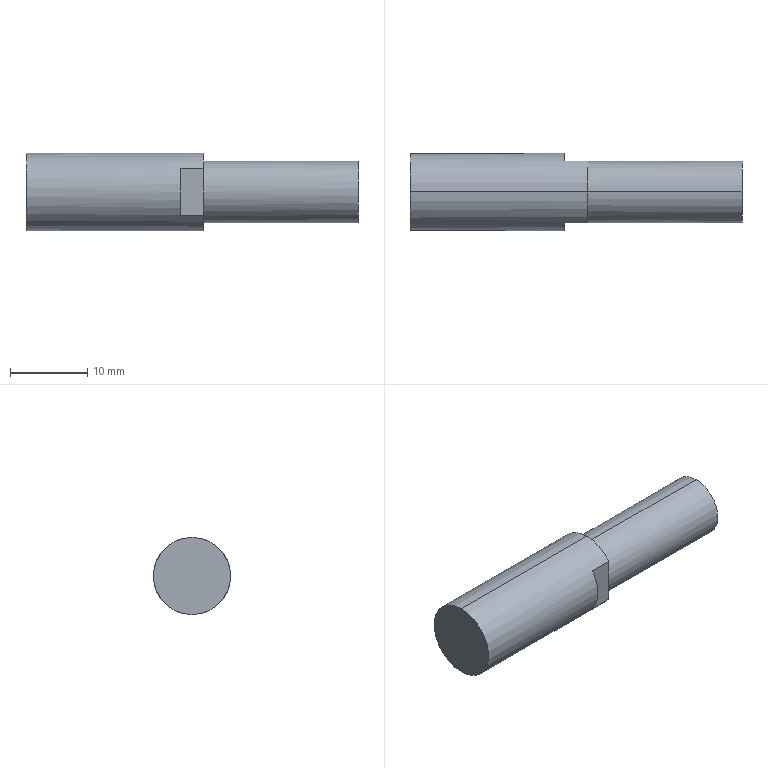Part | SolidWorks | features ICE 3, Extrusion 1 | 1 solid | 12 faces | box 43 x 10 x 10 mm | volume 2787 mm3 | plane 8 | cylinder 4 | commonest cylinder face diameters 8 x2 10 x2
STEP:
#1=CARTESIAN_POINT('',(20.,0.,-4.));
#2=VERTEX_POINT('',#1);
#3=CARTESIAN_POINT('',(20.,0.,4.));
#4=VERTEX_POINT('',#3);
#5=CARTESIAN_POINT('',(20.,0.,0.));
#6=DIRECTION('',(1.,0.,0.));
#7=DIRECTION('',(0.,0.,-1.));
#8=AXIS2_PLACEMENT_3D('',#5,#6,#7);
#9=CIRCLE('',#8,4.);
#10=EDGE_CURVE('',#2,#4,#9,.T.);
#11=ORIENTED_EDGE('',*,*,#10,.F.);
#12=CARTESIAN_POINT('',(0.,0.,-4.));
#13=VERTEX_POINT('',#12);
#14=CARTESIAN_POINT('',(20.,0.,-4.));
#15=DIRECTION('',(-1.,0.,0.));
#16=VECTOR('',#15,1000.);
#17=LINE('',#14,#16);
#18=EDGE_CURVE('',#2,#13,#17,.T.);
#19=ORIENTED_EDGE('',*,*,#18,.T.);
#20=CARTESIAN_POINT('',(0.,4.,0.));
#21=VERTEX_POINT('',#20);
#22=CARTESIAN_POINT('',(0.,0.,0.));
#23=DIRECTION('',(1.,0.,0.));
#24=DIRECTION('',(0.,0.,-1.));
#25=AXIS2_PLACEMENT_3D('',#22,#23,#24);
#26=CIRCLE('',#25,4.);
#27=EDGE_CURVE('',#13,#21,#26,.T.);
#28=ORIENTED_EDGE('',*,*,#27,.T.);
#29=CARTESIAN_POINT('',(0.,0.,4.));
#30=VERTEX_POINT('',#29);
#31=CARTESIAN_POINT('',(0.,0.,0.));
#32=DIRECTION('',(1.,0.,0.));
#33=DIRECTION('',(0.,0.,-1.));
#34=AXIS2_PLACEMENT_3D('',#31,#32,#33);
#35=CIRCLE('',#34,4.);
#36=EDGE_CURVE('',#21,#30,#35,.T.);
#37=ORIENTED_EDGE('',*,*,#36,.T.);
#38=CARTESIAN_POINT('',(20.,0.,4.));
#39=DIRECTION('',(-1.,0.,0.));
#40=VECTOR('',#39,1000.);
#41=LINE('',#38,#40);
#42=EDGE_CURVE('',#4,#30,#41,.T.);
#43=ORIENTED_EDGE('',*,*,#42,.F.);
#44=EDGE_LOOP('',(#11,#19,#28,#37,#43));
#45=FACE_OUTER_BOUND('',#44,.T.);
#46=CARTESIAN_POINT('',(20.,0.,0.));
#47=DIRECTION('',(-1.,0.,0.));
#48=DIRECTION('',(0.,0.,1.));
#49=AXIS2_PLACEMENT_3D('',#46,#47,#48);
#50=CYLINDRICAL_SURFACE('',#49,4.);
#51=ADVANCED_FACE('',(#45),#50,.T.);
#52=CARTESIAN_POINT('',(-23.,0.,5.));
#53=VERTEX_POINT('',#52);
#54=CARTESIAN_POINT('',(-23.,0.,-5.));
#55=VERTEX_POINT('',#54);
#56=CARTESIAN_POINT('',(-23.,0.,0.));
#57=DIRECTION('',(-1.,0.,0.));
#58=DIRECTION('',(0.,0.,1.));
#59=AXIS2_PLACEMENT_3D('',#56,#57,#58);
#60=CIRCLE('',#59,5.);
#61=EDGE_CURVE('',#53,#55,#60,.T.);
#62=ORIENTED_EDGE('',*,*,#61,.F.);
#63=CARTESIAN_POINT('',(0.,0.,5.));
#64=VERTEX_POINT('',#63);
#65=CARTESIAN_POINT('',(-3.,0.,5.));
#66=DIRECTION('',(1.,0.,0.));
#67=VECTOR('',#66,1000.);
#68=LINE('',#65,#67);
#69=EDGE_CURVE('',#53,#64,#68,.T.);
#70=ORIENTED_EDGE('',*,*,#69,.T.);
#71=CARTESIAN_POINT('',(0.,4.,3.));
#72=VERTEX_POINT('',#71);
#73=CARTESIAN_POINT('',(0.,0.,0.));
#74=DIRECTION('',(-1.,0.,0.));
#75=DIRECTION('',(0.,0.,1.));
#76=AXIS2_PLACEMENT_3D('',#73,#74,#75);
#77=CIRCLE('',#76,5.);
#78=EDGE_CURVE('',#64,#72,#77,.T.);
#79=ORIENTED_EDGE('',*,*,#78,.T.);
#80=CARTESIAN_POINT('',(-3.,4.,3.));
#81=VERTEX_POINT('',#80);
#82=CARTESIAN_POINT('',(-3.,4.,3.));
#83=DIRECTION('',(1.,0.,0.));
#84=VECTOR('',#83,1000.);
#85=LINE('',#82,#84);
#86=EDGE_CURVE('',#81,#72,#85,.T.);
#87=ORIENTED_EDGE('',*,*,#86,.F.);
#88=CARTESIAN_POINT('',(-3.,4.,-3.));
#89=VERTEX_POINT('',#88);
#90=CARTESIAN_POINT('',(-3.,0.,0.));
#91=DIRECTION('',(-1.,0.,0.));
#92=DIRECTION('',(0.,0.,1.));
#93=AXIS2_PLACEMENT_3D('',#90,#91,#92);
#94=CIRCLE('',#93,5.);
#95=EDGE_CURVE('',#81,#89,#94,.T.);
#96=ORIENTED_EDGE('',*,*,#95,.T.);
#97=CARTESIAN_POINT('',(0.,4.,-3.));
#98=VERTEX_POINT('',#97);
#99=CARTESIAN_POINT('',(-3.,4.,-3.));
#100=DIRECTION('',(-1.,0.,0.));
#101=VECTOR('',#100,1000.);
#102=LINE('',#99,#101);
#103=EDGE_CURVE('',#98,#89,#102,.T.);
#104=ORIENTED_EDGE('',*,*,#103,.F.);
#105=CARTESIAN_POINT('',(0.,0.,-5.));
#106=VERTEX_POINT('',#105);
#107=CARTESIAN_POINT('',(0.,0.,0.));
#108=DIRECTION('',(-1.,0.,0.));
#109=DIRECTION('',(0.,0.,1.));
#110=AXIS2_PLACEMENT_3D('',#107,#108,#109);
#111=CIRCLE('',#110,5.);
#112=EDGE_CURVE('',#98,#106,#111,.T.);
#113=ORIENTED_EDGE('',*,*,#112,.T.);
#114=CARTESIAN_POINT('',(-3.,0.,-5.));
#115=DIRECTION('',(1.,0.,0.));
#116=VECTOR('',#115,1000.);
#117=LINE('',#114,#116);
#118=EDGE_CURVE('',#55,#106,#117,.T.);
#119=ORIENTED_EDGE('',*,*,#118,.F.);
#120=EDGE_LOOP('',(#62,#70,#79,#87,#96,#104,#113,#119));
#121=FACE_OUTER_BOUND('',#120,.T.);
#122=CARTESIAN_POINT('',(-3.,0.,0.));
#123=DIRECTION('',(1.,0.,0.));
#124=DIRECTION('',(0.,0.,-1.));
#125=AXIS2_PLACEMENT_3D('',#122,#123,#124);
#126=CYLINDRICAL_SURFACE('',#125,5.);
#127=ADVANCED_FACE('',(#121),#126,.T.);
#128=ORIENTED_EDGE('',*,*,#69,.F.);
#129=CARTESIAN_POINT('',(-23.,0.,0.));
#130=DIRECTION('',(-1.,0.,0.));
#131=DIRECTION('',(0.,0.,1.));
#132=AXIS2_PLACEMENT_3D('',#129,#130,#131);
#133=CIRCLE('',#132,5.);
#134=EDGE_CURVE('',#55,#53,#133,.T.);
#135=ORIENTED_EDGE('',*,*,#134,.F.);
#136=ORIENTED_EDGE('',*,*,#118,.T.);
#137=CARTESIAN_POINT('',(0.,-4.,-3.));
#138=VERTEX_POINT('',#137);
#139=CARTESIAN_POINT('',(0.,0.,0.));
#140=DIRECTION('',(-1.,0.,0.));
#141=DIRECTION('',(0.,0.,1.));
#142=AXIS2_PLACEMENT_3D('',#139,#140,#141);
#143=CIRCLE('',#142,5.);
#144=EDGE_CURVE('',#106,#138,#143,.T.);
#145=ORIENTED_EDGE('',*,*,#144,.T.);
#146=CARTESIAN_POINT('',(-3.,-4.,-3.));
#147=VERTEX_POINT('',#146);
#148=CARTESIAN_POINT('',(-3.,-4.,-3.));
#149=DIRECTION('',(1.,0.,0.));
#150=VECTOR('',#149,1000.);
#151=LINE('',#148,#150);
#152=EDGE_CURVE('',#147,#138,#151,.T.);
#153=ORIENTED_EDGE('',*,*,#152,.F.);
#154=CARTESIAN_POINT('',(-3.,-4.,3.));
#155=VERTEX_POINT('',#154);
#156=CARTESIAN_POINT('',(-3.,0.,0.));
#157=DIRECTION('',(-1.,0.,0.));
#158=DIRECTION('',(0.,0.,1.));
#159=AXIS2_PLACEMENT_3D('',#156,#157,#158);
#160=CIRCLE('',#159,5.);
#161=EDGE_CURVE('',#147,#155,#160,.T.);
#162=ORIENTED_EDGE('',*,*,#161,.T.);
#163=CARTESIAN_POINT('',(0.,-4.,3.));
#164=VERTEX_POINT('',#163);
#165=CARTESIAN_POINT('',(-3.,-4.,3.));
#166=DIRECTION('',(-1.,0.,0.));
#167=VECTOR('',#166,1000.);
#168=LINE('',#165,#167);
#169=EDGE_CURVE('',#164,#155,#168,.T.);
#170=ORIENTED_EDGE('',*,*,#169,.F.);
#171=CARTESIAN_POINT('',(0.,0.,0.));
#172=DIRECTION('',(-1.,0.,0.));
#173=DIRECTION('',(0.,0.,1.));
#174=AXIS2_PLACEMENT_3D('',#171,#172,#173);
#175=CIRCLE('',#174,5.);
#176=EDGE_CURVE('',#164,#64,#175,.T.);
#177=ORIENTED_EDGE('',*,*,#176,.T.);
#178=EDGE_LOOP('',(#128,#135,#136,#145,#153,#162,#170,#177));
#179=FACE_OUTER_BOUND('',#178,.T.);
#180=CARTESIAN_POINT('',(-3.,0.,0.));
#181=DIRECTION('',(1.,0.,0.));
#182=DIRECTION('',(0.,0.,-1.));
#183=AXIS2_PLACEMENT_3D('',#180,#181,#182);
#184=CYLINDRICAL_SURFACE('',#183,5.);
#185=ADVANCED_FACE('',(#179),#184,.T.);
#186=CARTESIAN_POINT('',(0.,-4.,0.));
#187=VERTEX_POINT('',#186);
#188=CARTESIAN_POINT('',(0.,-4.,0.));
#189=DIRECTION('',(0.,0.,1.));
#190=VECTOR('',#189,1000.);
#191=LINE('',#188,#190);
#192=EDGE_CURVE('',#138,#187,#191,.T.);
#193=ORIENTED_EDGE('',*,*,#192,.F.);
#194=ORIENTED_EDGE('',*,*,#144,.F.);
#195=ORIENTED_EDGE('',*,*,#112,.F.);
#196=CARTESIAN_POINT('',(0.,4.,0.));
#197=DIRECTION('',(0.,0.,-1.));
#198=VECTOR('',#197,1000.);
#199=LINE('',#196,#198);
#200=EDGE_CURVE('',#21,#98,#199,.T.);
#201=ORIENTED_EDGE('',*,*,#200,.F.);
#202=ORIENTED_EDGE('',*,*,#27,.F.);
#203=CARTESIAN_POINT('',(0.,0.,0.));
#204=DIRECTION('',(1.,0.,0.));
#205=DIRECTION('',(0.,0.,-1.));
#206=AXIS2_PLACEMENT_3D('',#203,#204,#205);
#207=CIRCLE('',#206,4.);
#208=EDGE_CURVE('',#187,#13,#207,.T.);
#209=ORIENTED_EDGE('',*,*,#208,.F.);
#210=EDGE_LOOP('',(#193,#194,#195,#201,#202,#209));
#211=FACE_OUTER_BOUND('',#210,.T.);
#212=CARTESIAN_POINT('',(0.,0.,0.));
#213=DIRECTION('',(-1.,0.,0.));
#214=DIRECTION('',(0.,0.,1.));
#215=AXIS2_PLACEMENT_3D('',#212,#213,#214);
#216=PLANE('',#215);
#217=ADVANCED_FACE('',(#211),#216,.F.);
#218=CARTESIAN_POINT('',(0.,-4.,0.));
#219=DIRECTION('',(0.,0.,1.));
#220=VECTOR('',#219,1000.);
#221=LINE('',#218,#220);
#222=EDGE_CURVE('',#187,#164,#221,.T.);
#223=ORIENTED_EDGE('',*,*,#222,.F.);
#224=CARTESIAN_POINT('',(0.,0.,0.));
#225=DIRECTION('',(1.,0.,0.));
#226=DIRECTION('',(0.,0.,-1.));
#227=AXIS2_PLACEMENT_3D('',#224,#225,#226);
#228=CIRCLE('',#227,4.);
#229=EDGE_CURVE('',#30,#187,#228,.T.);
#230=ORIENTED_EDGE('',*,*,#229,.F.);
#231=ORIENTED_EDGE('',*,*,#36,.F.);
#232=CARTESIAN_POINT('',(0.,4.,0.));
#233=DIRECTION('',(0.,0.,-1.));
#234=VECTOR('',#233,1000.);
#235=LINE('',#232,#234);
#236=EDGE_CURVE('',#72,#21,#235,.T.);
#237=ORIENTED_EDGE('',*,*,#236,.F.);
#238=ORIENTED_EDGE('',*,*,#78,.F.);
#239=ORIENTED_EDGE('',*,*,#176,.F.);
#240=EDGE_LOOP('',(#223,#230,#231,#237,#238,#239));
#241=FACE_OUTER_BOUND('',#240,.T.);
#242=CARTESIAN_POINT('',(0.,0.,0.));
#243=DIRECTION('',(-1.,0.,0.));
#244=DIRECTION('',(0.,0.,1.));
#245=AXIS2_PLACEMENT_3D('',#242,#243,#244);
#246=PLANE('',#245);
#247=ADVANCED_FACE('',(#241),#246,.F.);
#248=ORIENTED_EDGE('',*,*,#18,.F.);
#249=CARTESIAN_POINT('',(20.,0.,0.));
#250=DIRECTION('',(1.,0.,0.));
#251=DIRECTION('',(0.,0.,-1.));
#252=AXIS2_PLACEMENT_3D('',#249,#250,#251);
#253=CIRCLE('',#252,4.);
#254=EDGE_CURVE('',#4,#2,#253,.T.);
#255=ORIENTED_EDGE('',*,*,#254,.F.);
#256=ORIENTED_EDGE('',*,*,#42,.T.);
#257=ORIENTED_EDGE('',*,*,#229,.T.);
#258=ORIENTED_EDGE('',*,*,#208,.T.);
#259=EDGE_LOOP('',(#248,#255,#256,#257,#258));
#260=FACE_OUTER_BOUND('',#259,.T.);
#261=CARTESIAN_POINT('',(20.,0.,0.));
#262=DIRECTION('',(-1.,0.,0.));
#263=DIRECTION('',(0.,0.,1.));
#264=AXIS2_PLACEMENT_3D('',#261,#262,#263);
#265=CYLINDRICAL_SURFACE('',#264,4.);
#266=ADVANCED_FACE('',(#260),#265,.T.);
#267=ORIENTED_EDGE('',*,*,#254,.T.);
#268=ORIENTED_EDGE('',*,*,#10,.T.);
#269=EDGE_LOOP('',(#267,#268));
#270=FACE_OUTER_BOUND('',#269,.T.);
#271=CARTESIAN_POINT('',(20.,0.,0.));
#272=DIRECTION('',(1.,0.,0.));
#273=DIRECTION('',(0.,0.,-1.));
#274=AXIS2_PLACEMENT_3D('',#271,#272,#273);
#275=PLANE('',#274);
#276=ADVANCED_FACE('',(#270),#275,.T.);
#277=ORIENTED_EDGE('',*,*,#86,.T.);
#278=ORIENTED_EDGE('',*,*,#236,.T.);
#279=ORIENTED_EDGE('',*,*,#200,.T.);
#280=ORIENTED_EDGE('',*,*,#103,.T.);
#281=CARTESIAN_POINT('',(-3.,4.,-7.087));
#282=DIRECTION('',(0.,0.,-1.));
#283=VECTOR('',#282,1000.);
#284=LINE('',#281,#283);
#285=EDGE_CURVE('',#81,#89,#284,.T.);
#286=ORIENTED_EDGE('',*,*,#285,.F.);
#287=EDGE_LOOP('',(#277,#278,#279,#280,#286));
#288=FACE_OUTER_BOUND('',#287,.T.);
#289=CARTESIAN_POINT('',(20.,4.,-7.087));
#290=DIRECTION('',(0.,1.,0.));
#291=DIRECTION('',(0.,0.,1.));
#292=AXIS2_PLACEMENT_3D('',#289,#290,#291);
#293=PLANE('',#292);
#294=ADVANCED_FACE('',(#288),#293,.T.);
#295=ORIENTED_EDGE('',*,*,#152,.T.);
#296=ORIENTED_EDGE('',*,*,#192,.T.);
#297=ORIENTED_EDGE('',*,*,#222,.T.);
#298=ORIENTED_EDGE('',*,*,#169,.T.);
#299=CARTESIAN_POINT('',(-3.,-4.,-7.087));
#300=DIRECTION('',(0.,0.,1.));
#301=VECTOR('',#300,1000.);
#302=LINE('',#299,#301);
#303=EDGE_CURVE('',#147,#155,#302,.T.);
#304=ORIENTED_EDGE('',*,*,#303,.F.);
#305=EDGE_LOOP('',(#295,#296,#297,#298,#304));
#306=FACE_OUTER_BOUND('',#305,.T.);
#307=CARTESIAN_POINT('',(20.,-4.,-7.087));
#308=DIRECTION('',(0.,-1.,0.));
#309=DIRECTION('',(0.,0.,-1.));
#310=AXIS2_PLACEMENT_3D('',#307,#308,#309);
#311=PLANE('',#310);
#312=ADVANCED_FACE('',(#306),#311,.T.);
#313=ORIENTED_EDGE('',*,*,#161,.F.);
#314=ORIENTED_EDGE('',*,*,#303,.T.);
#315=EDGE_LOOP('',(#313,#314));
#316=FACE_OUTER_BOUND('',#315,.T.);
#317=CARTESIAN_POINT('',(-3.,0.,0.));
#318=DIRECTION('',(-1.,0.,0.));
#319=DIRECTION('',(0.,0.,1.));
#320=AXIS2_PLACEMENT_3D('',#317,#318,#319);
#321=PLANE('',#320);
#322=ADVANCED_FACE('',(#316),#321,.F.);
#323=ORIENTED_EDGE('',*,*,#95,.F.);
#324=ORIENTED_EDGE('',*,*,#285,.T.);
#325=EDGE_LOOP('',(#323,#324));
#326=FACE_OUTER_BOUND('',#325,.T.);
#327=CARTESIAN_POINT('',(-3.,0.,0.));
#328=DIRECTION('',(-1.,0.,0.));
#329=DIRECTION('',(0.,0.,1.));
#330=AXIS2_PLACEMENT_3D('',#327,#328,#329);
#331=PLANE('',#330);
#332=ADVANCED_FACE('',(#326),#331,.F.);
#333=ORIENTED_EDGE('',*,*,#134,.T.);
#334=ORIENTED_EDGE('',*,*,#61,.T.);
#335=EDGE_LOOP('',(#333,#334));
#336=FACE_OUTER_BOUND('',#335,.T.);
#337=CARTESIAN_POINT('',(-23.,0.,0.));
#338=DIRECTION('',(-1.,0.,0.));
#339=DIRECTION('',(0.,0.,1.));
#340=AXIS2_PLACEMENT_3D('',#337,#338,#339);
#341=PLANE('',#340);
#342=ADVANCED_FACE('',(#336),#341,.T.);
#343=CLOSED_SHELL('',(#51,#127,#185,#217,#247,#266,#276,#294,#312,#322,#332,#342));
#344=MANIFOLD_SOLID_BREP('',#343);
#345=CARTESIAN_POINT('',(0.,0.,0.));
#346=DIRECTION('',(0.,0.,1.));
#347=DIRECTION('',(1.,0.,0.));
#348=AXIS2_PLACEMENT_3D('',#345,#346,#347);
#349=(LENGTH_UNIT()NAMED_UNIT(*)SI_UNIT(.MILLI.,.METRE.));
#350=UNCERTAINTY_MEASURE_WITH_UNIT(LENGTH_MEASURE(0.00001),#349,'','');
#351=(NAMED_UNIT(*)PLANE_ANGLE_UNIT()SI_UNIT($,.RADIAN.));
#352=(NAMED_UNIT(*)SI_UNIT($,.STERADIAN.)SOLID_ANGLE_UNIT());
#353=(GEOMETRIC_REPRESENTATION_CONTEXT(3)GLOBAL_UNCERTAINTY_ASSIGNED_CONTEXT((#350))GLOBAL_UNIT_ASSIGNED_CONTEXT((#349,#351,#352))REPRESENTATION_CONTEXT('',''));
#354=ADVANCED_BREP_SHAPE_REPRESENTATION('',(#344,#348),#353);